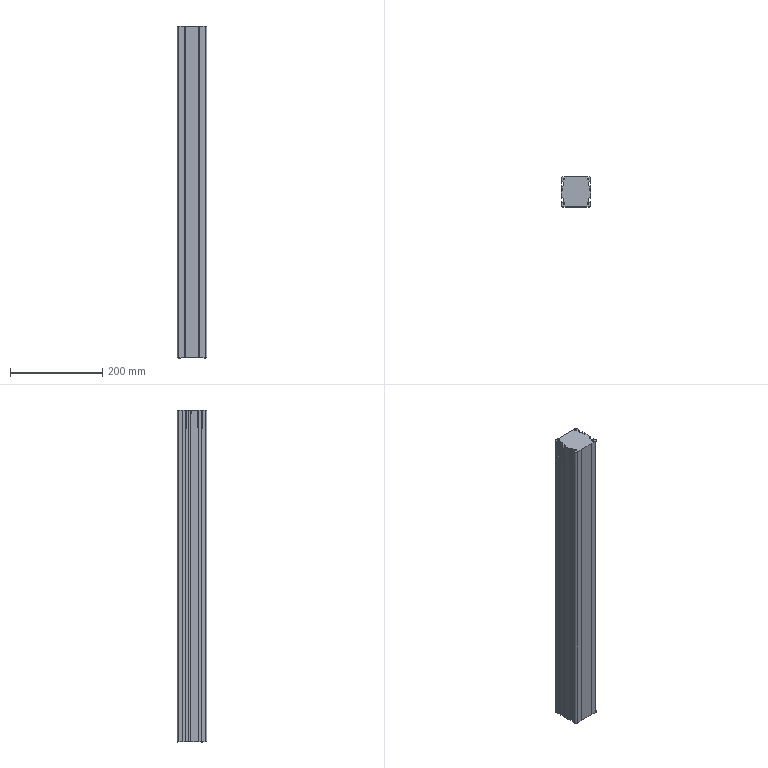Part | SolidWorks | features BaseBody 1 | 1 solid | 194 faces | box 65 x 65 x 720 mm | volume 2838677 mm3 | cylinder 96 | plane 82 | cone 16 | commonest cylinder face diameters 0.6 x48 4.2 x16 1 x12 3 x12 2 x4 8 x4